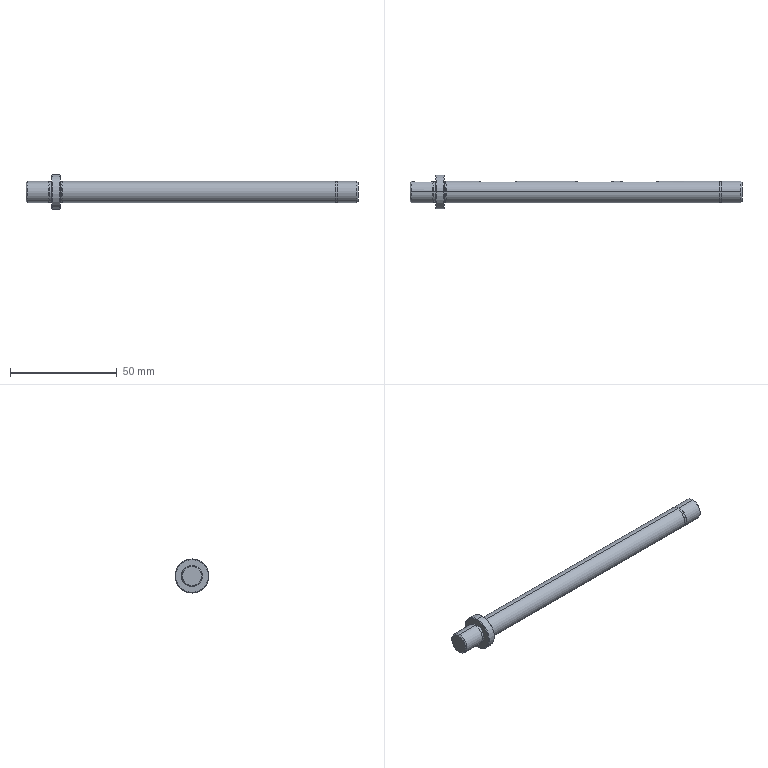Part | SolidWorks | features ICE 9, Chamfer 6, Extrusion 1, RefAxis 1 | 1 solid | 53 faces | box 155.5 x 16 x 16 mm | volume 12095 mm3 | cylinder 22 | plane 18 | cone 13 | commonest cylinder face diameters 4 x8 10 x6 9.5 x4 9.6 x2 16 x2